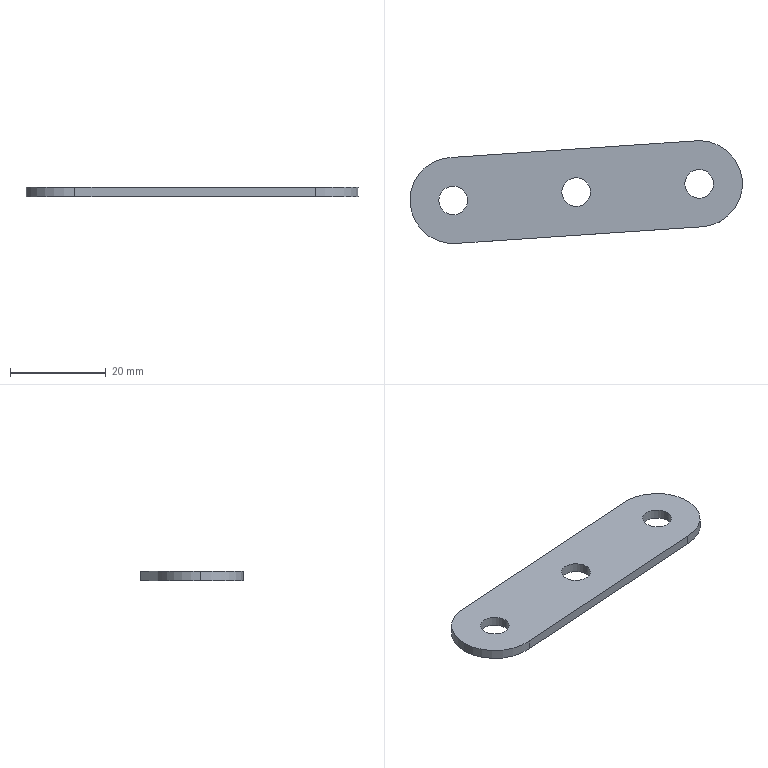Part | SolidWorks | features Extrusion 1 | 1 solid | 13 faces | box 69.294 x 21.478 x 2 mm | volume 2186 mm3 | cylinder 9 | plane 4 | commonest cylinder face diameters 6 x6 18 x3
STEP:
#1=CARTESIAN_POINT('',(-28.647,-1.739,2.));
#2=VERTEX_POINT('',#1);
#3=CARTESIAN_POINT('',(-22.647,-1.739,2.));
#4=VERTEX_POINT('',#3);
#5=CARTESIAN_POINT('',(-25.647,-1.739,2.));
#6=DIRECTION('',(0.,0.,1.));
#7=DIRECTION('',(1.,0.,0.));
#8=AXIS2_PLACEMENT_3D('',#5,#6,#7);
#9=CIRCLE('',#8,3.);
#10=EDGE_CURVE('',#2,#4,#9,.T.);
#11=ORIENTED_EDGE('',*,*,#10,.T.);
#12=CARTESIAN_POINT('',(-22.647,-1.739,0.));
#13=VERTEX_POINT('',#12);
#14=CARTESIAN_POINT('',(-22.647,-1.739,2.));
#15=DIRECTION('',(0.,0.,-1.));
#16=VECTOR('',#15,1000.);
#17=LINE('',#14,#16);
#18=EDGE_CURVE('',#4,#13,#17,.T.);
#19=ORIENTED_EDGE('',*,*,#18,.T.);
#20=CARTESIAN_POINT('',(-28.647,-1.739,0.));
#21=VERTEX_POINT('',#20);
#22=CARTESIAN_POINT('',(-25.647,-1.739,0.));
#23=DIRECTION('',(0.,0.,1.));
#24=DIRECTION('',(1.,0.,0.));
#25=AXIS2_PLACEMENT_3D('',#22,#23,#24);
#26=CIRCLE('',#25,3.);
#27=EDGE_CURVE('',#21,#13,#26,.T.);
#28=ORIENTED_EDGE('',*,*,#27,.F.);
#29=CARTESIAN_POINT('',(-28.647,-1.739,2.));
#30=DIRECTION('',(0.,0.,-1.));
#31=VECTOR('',#30,1000.);
#32=LINE('',#29,#31);
#33=EDGE_CURVE('',#2,#21,#32,.T.);
#34=ORIENTED_EDGE('',*,*,#33,.F.);
#35=EDGE_LOOP('',(#11,#19,#28,#34));
#36=FACE_OUTER_BOUND('',#35,.T.);
#37=CARTESIAN_POINT('',(-25.647,-1.739,2.));
#38=DIRECTION('',(0.,0.,-1.));
#39=DIRECTION('',(-1.,0.,0.));
#40=AXIS2_PLACEMENT_3D('',#37,#38,#39);
#41=CYLINDRICAL_SURFACE('',#40,3.);
#42=ADVANCED_FACE('',(#36),#41,.F.);
#43=CARTESIAN_POINT('',(-3.,0.,2.));
#44=VERTEX_POINT('',#43);
#45=CARTESIAN_POINT('',(3.,0.,2.));
#46=VERTEX_POINT('',#45);
#47=CARTESIAN_POINT('',(0.,0.,2.));
#48=DIRECTION('',(0.,0.,1.));
#49=DIRECTION('',(1.,0.,0.));
#50=AXIS2_PLACEMENT_3D('',#47,#48,#49);
#51=CIRCLE('',#50,3.);
#52=EDGE_CURVE('',#44,#46,#51,.T.);
#53=ORIENTED_EDGE('',*,*,#52,.T.);
#54=CARTESIAN_POINT('',(3.,0.,0.));
#55=VERTEX_POINT('',#54);
#56=CARTESIAN_POINT('',(3.,0.,2.));
#57=DIRECTION('',(0.,0.,-1.));
#58=VECTOR('',#57,1000.);
#59=LINE('',#56,#58);
#60=EDGE_CURVE('',#46,#55,#59,.T.);
#61=ORIENTED_EDGE('',*,*,#60,.T.);
#62=CARTESIAN_POINT('',(-3.,0.,0.));
#63=VERTEX_POINT('',#62);
#64=CARTESIAN_POINT('',(0.,0.,0.));
#65=DIRECTION('',(0.,0.,1.));
#66=DIRECTION('',(1.,0.,0.));
#67=AXIS2_PLACEMENT_3D('',#64,#65,#66);
#68=CIRCLE('',#67,3.);
#69=EDGE_CURVE('',#63,#55,#68,.T.);
#70=ORIENTED_EDGE('',*,*,#69,.F.);
#71=CARTESIAN_POINT('',(-3.,0.,2.));
#72=DIRECTION('',(0.,0.,-1.));
#73=VECTOR('',#72,1000.);
#74=LINE('',#71,#73);
#75=EDGE_CURVE('',#44,#63,#74,.T.);
#76=ORIENTED_EDGE('',*,*,#75,.F.);
#77=EDGE_LOOP('',(#53,#61,#70,#76));
#78=FACE_OUTER_BOUND('',#77,.T.);
#79=CARTESIAN_POINT('',(0.,0.,2.));
#80=DIRECTION('',(0.,0.,-1.));
#81=DIRECTION('',(-1.,0.,0.));
#82=AXIS2_PLACEMENT_3D('',#79,#80,#81);
#83=CYLINDRICAL_SURFACE('',#82,3.);
#84=ADVANCED_FACE('',(#78),#83,.F.);
#85=CARTESIAN_POINT('',(-54.294,-3.478,2.));
#86=VERTEX_POINT('',#85);
#87=CARTESIAN_POINT('',(-48.294,-3.478,2.));
#88=VERTEX_POINT('',#87);
#89=CARTESIAN_POINT('',(-51.294,-3.478,2.));
#90=DIRECTION('',(0.,0.,1.));
#91=DIRECTION('',(1.,0.,0.));
#92=AXIS2_PLACEMENT_3D('',#89,#90,#91);
#93=CIRCLE('',#92,3.);
#94=EDGE_CURVE('',#86,#88,#93,.T.);
#95=ORIENTED_EDGE('',*,*,#94,.T.);
#96=CARTESIAN_POINT('',(-48.294,-3.478,0.));
#97=VERTEX_POINT('',#96);
#98=CARTESIAN_POINT('',(-48.294,-3.478,2.));
#99=DIRECTION('',(0.,0.,-1.));
#100=VECTOR('',#99,1000.);
#101=LINE('',#98,#100);
#102=EDGE_CURVE('',#88,#97,#101,.T.);
#103=ORIENTED_EDGE('',*,*,#102,.T.);
#104=CARTESIAN_POINT('',(-54.294,-3.478,0.));
#105=VERTEX_POINT('',#104);
#106=CARTESIAN_POINT('',(-51.294,-3.478,0.));
#107=DIRECTION('',(0.,0.,1.));
#108=DIRECTION('',(1.,0.,0.));
#109=AXIS2_PLACEMENT_3D('',#106,#107,#108);
#110=CIRCLE('',#109,3.);
#111=EDGE_CURVE('',#105,#97,#110,.T.);
#112=ORIENTED_EDGE('',*,*,#111,.F.);
#113=CARTESIAN_POINT('',(-54.294,-3.478,2.));
#114=DIRECTION('',(0.,0.,-1.));
#115=VECTOR('',#114,1000.);
#116=LINE('',#113,#115);
#117=EDGE_CURVE('',#86,#105,#116,.T.);
#118=ORIENTED_EDGE('',*,*,#117,.F.);
#119=EDGE_LOOP('',(#95,#103,#112,#118));
#120=FACE_OUTER_BOUND('',#119,.T.);
#121=CARTESIAN_POINT('',(-51.294,-3.478,2.));
#122=DIRECTION('',(0.,0.,-1.));
#123=DIRECTION('',(-1.,0.,0.));
#124=AXIS2_PLACEMENT_3D('',#121,#122,#123);
#125=CYLINDRICAL_SURFACE('',#124,3.);
#126=ADVANCED_FACE('',(#120),#125,.F.);
#127=CARTESIAN_POINT('',(-60.294,-3.478,2.));
#128=VERTEX_POINT('',#127);
#129=CARTESIAN_POINT('',(-50.079,-12.396,2.));
#130=VERTEX_POINT('',#129);
#131=CARTESIAN_POINT('',(-51.294,-3.478,2.));
#132=DIRECTION('',(0.,0.,1.));
#133=DIRECTION('',(1.,0.,0.));
#134=AXIS2_PLACEMENT_3D('',#131,#132,#133);
#135=CIRCLE('',#134,9.);
#136=EDGE_CURVE('',#128,#130,#135,.T.);
#137=ORIENTED_EDGE('',*,*,#136,.F.);
#138=CARTESIAN_POINT('',(-60.294,-3.478,0.));
#139=VERTEX_POINT('',#138);
#140=CARTESIAN_POINT('',(-60.294,-3.478,2.));
#141=DIRECTION('',(0.,0.,-1.));
#142=VECTOR('',#141,1000.);
#143=LINE('',#140,#142);
#144=EDGE_CURVE('',#128,#139,#143,.T.);
#145=ORIENTED_EDGE('',*,*,#144,.T.);
#146=CARTESIAN_POINT('',(-50.079,-12.396,0.));
#147=VERTEX_POINT('',#146);
#148=CARTESIAN_POINT('',(-51.294,-3.478,0.));
#149=DIRECTION('',(0.,0.,1.));
#150=DIRECTION('',(1.,0.,0.));
#151=AXIS2_PLACEMENT_3D('',#148,#149,#150);
#152=CIRCLE('',#151,9.);
#153=EDGE_CURVE('',#139,#147,#152,.T.);
#154=ORIENTED_EDGE('',*,*,#153,.T.);
#155=CARTESIAN_POINT('',(-50.079,-12.396,2.));
#156=DIRECTION('',(0.,0.,-1.));
#157=VECTOR('',#156,1000.);
#158=LINE('',#155,#157);
#159=EDGE_CURVE('',#130,#147,#158,.T.);
#160=ORIENTED_EDGE('',*,*,#159,.F.);
#161=EDGE_LOOP('',(#137,#145,#154,#160));
#162=FACE_OUTER_BOUND('',#161,.T.);
#163=CARTESIAN_POINT('',(-51.294,-3.478,2.));
#164=DIRECTION('',(0.,0.,-1.));
#165=DIRECTION('',(-1.,0.,0.));
#166=AXIS2_PLACEMENT_3D('',#163,#164,#165);
#167=CYLINDRICAL_SURFACE('',#166,9.);
#168=ADVANCED_FACE('',(#162),#167,.T.);
#169=ORIENTED_EDGE('',*,*,#52,.F.);
#170=CARTESIAN_POINT('',(0.,0.,2.));
#171=DIRECTION('',(0.,0.,1.));
#172=DIRECTION('',(1.,0.,0.));
#173=AXIS2_PLACEMENT_3D('',#170,#171,#172);
#174=CIRCLE('',#173,3.);
#175=EDGE_CURVE('',#46,#44,#174,.T.);
#176=ORIENTED_EDGE('',*,*,#175,.F.);
#177=EDGE_LOOP('',(#169,#176));
#178=FACE_BOUND('',#177,.T.);
#179=CARTESIAN_POINT('',(-51.294,5.522,2.));
#180=VERTEX_POINT('',#179);
#181=CARTESIAN_POINT('',(-51.294,-3.478,2.));
#182=DIRECTION('',(0.,0.,1.));
#183=DIRECTION('',(1.,0.,0.));
#184=AXIS2_PLACEMENT_3D('',#181,#182,#183);
#185=CIRCLE('',#184,9.);
#186=EDGE_CURVE('',#180,#128,#185,.T.);
#187=ORIENTED_EDGE('',*,*,#186,.T.);
#188=ORIENTED_EDGE('',*,*,#136,.T.);
#189=CARTESIAN_POINT('',(0.,-9.,2.));
#190=VERTEX_POINT('',#189);
#191=CARTESIAN_POINT('',(-50.079,-12.396,2.));
#192=DIRECTION('',(0.9977,0.06765,0.));
#193=VECTOR('',#192,1000.);
#194=LINE('',#191,#193);
#195=EDGE_CURVE('',#130,#190,#194,.T.);
#196=ORIENTED_EDGE('',*,*,#195,.T.);
#197=CARTESIAN_POINT('',(0.,9.,2.));
#198=VERTEX_POINT('',#197);
#199=CARTESIAN_POINT('',(0.,0.,2.));
#200=DIRECTION('',(0.,0.,1.));
#201=DIRECTION('',(1.,0.,0.));
#202=AXIS2_PLACEMENT_3D('',#199,#200,#201);
#203=CIRCLE('',#202,9.);
#204=EDGE_CURVE('',#190,#198,#203,.T.);
#205=ORIENTED_EDGE('',*,*,#204,.T.);
#206=CARTESIAN_POINT('',(-51.294,5.522,2.));
#207=DIRECTION('',(-0.9977,-0.06765,0.));
#208=VECTOR('',#207,1000.);
#209=LINE('',#206,#208);
#210=EDGE_CURVE('',#198,#180,#209,.T.);
#211=ORIENTED_EDGE('',*,*,#210,.T.);
#212=EDGE_LOOP('',(#187,#188,#196,#205,#211));
#213=FACE_OUTER_BOUND('',#212,.T.);
#214=ORIENTED_EDGE('',*,*,#94,.F.);
#215=CARTESIAN_POINT('',(-51.294,-3.478,2.));
#216=DIRECTION('',(0.,0.,1.));
#217=DIRECTION('',(1.,0.,0.));
#218=AXIS2_PLACEMENT_3D('',#215,#216,#217);
#219=CIRCLE('',#218,3.);
#220=EDGE_CURVE('',#88,#86,#219,.T.);
#221=ORIENTED_EDGE('',*,*,#220,.F.);
#222=EDGE_LOOP('',(#214,#221));
#223=FACE_BOUND('',#222,.T.);
#224=ORIENTED_EDGE('',*,*,#10,.F.);
#225=CARTESIAN_POINT('',(-25.647,-1.739,2.));
#226=DIRECTION('',(0.,0.,1.));
#227=DIRECTION('',(1.,0.,0.));
#228=AXIS2_PLACEMENT_3D('',#225,#226,#227);
#229=CIRCLE('',#228,3.);
#230=EDGE_CURVE('',#4,#2,#229,.T.);
#231=ORIENTED_EDGE('',*,*,#230,.F.);
#232=EDGE_LOOP('',(#224,#231));
#233=FACE_BOUND('',#232,.T.);
#234=CARTESIAN_POINT('',(-51.294,-3.478,2.));
#235=DIRECTION('',(0.,0.,1.));
#236=DIRECTION('',(1.,0.,0.));
#237=AXIS2_PLACEMENT_3D('',#234,#235,#236);
#238=PLANE('',#237);
#239=ADVANCED_FACE('',(#178,#213,#223,#233),#238,.T.);
#240=CARTESIAN_POINT('',(-51.294,5.522,0.));
#241=VERTEX_POINT('',#240);
#242=CARTESIAN_POINT('',(-51.294,-3.478,0.));
#243=DIRECTION('',(0.,0.,1.));
#244=DIRECTION('',(1.,0.,0.));
#245=AXIS2_PLACEMENT_3D('',#242,#243,#244);
#246=CIRCLE('',#245,9.);
#247=EDGE_CURVE('',#241,#139,#246,.T.);
#248=ORIENTED_EDGE('',*,*,#247,.F.);
#249=CARTESIAN_POINT('',(0.,9.,0.));
#250=VERTEX_POINT('',#249);
#251=CARTESIAN_POINT('',(-51.294,5.522,0.));
#252=DIRECTION('',(-0.9977,-0.06765,0.));
#253=VECTOR('',#252,1000.);
#254=LINE('',#251,#253);
#255=EDGE_CURVE('',#250,#241,#254,.T.);
#256=ORIENTED_EDGE('',*,*,#255,.F.);
#257=CARTESIAN_POINT('',(0.,-9.,0.));
#258=VERTEX_POINT('',#257);
#259=CARTESIAN_POINT('',(0.,0.,0.));
#260=DIRECTION('',(0.,0.,1.));
#261=DIRECTION('',(1.,0.,0.));
#262=AXIS2_PLACEMENT_3D('',#259,#260,#261);
#263=CIRCLE('',#262,9.);
#264=EDGE_CURVE('',#258,#250,#263,.T.);
#265=ORIENTED_EDGE('',*,*,#264,.F.);
#266=CARTESIAN_POINT('',(-50.079,-12.396,0.));
#267=DIRECTION('',(0.9977,0.06765,0.));
#268=VECTOR('',#267,1000.);
#269=LINE('',#266,#268);
#270=EDGE_CURVE('',#147,#258,#269,.T.);
#271=ORIENTED_EDGE('',*,*,#270,.F.);
#272=ORIENTED_EDGE('',*,*,#153,.F.);
#273=EDGE_LOOP('',(#248,#256,#265,#271,#272));
#274=FACE_OUTER_BOUND('',#273,.T.);
#275=ORIENTED_EDGE('',*,*,#111,.T.);
#276=CARTESIAN_POINT('',(-51.294,-3.478,0.));
#277=DIRECTION('',(0.,0.,1.));
#278=DIRECTION('',(1.,0.,0.));
#279=AXIS2_PLACEMENT_3D('',#276,#277,#278);
#280=CIRCLE('',#279,3.);
#281=EDGE_CURVE('',#97,#105,#280,.T.);
#282=ORIENTED_EDGE('',*,*,#281,.T.);
#283=EDGE_LOOP('',(#275,#282));
#284=FACE_BOUND('',#283,.T.);
#285=ORIENTED_EDGE('',*,*,#69,.T.);
#286=CARTESIAN_POINT('',(0.,0.,0.));
#287=DIRECTION('',(0.,0.,1.));
#288=DIRECTION('',(1.,0.,0.));
#289=AXIS2_PLACEMENT_3D('',#286,#287,#288);
#290=CIRCLE('',#289,3.);
#291=EDGE_CURVE('',#55,#63,#290,.T.);
#292=ORIENTED_EDGE('',*,*,#291,.T.);
#293=EDGE_LOOP('',(#285,#292));
#294=FACE_BOUND('',#293,.T.);
#295=ORIENTED_EDGE('',*,*,#27,.T.);
#296=CARTESIAN_POINT('',(-25.647,-1.739,0.));
#297=DIRECTION('',(0.,0.,1.));
#298=DIRECTION('',(1.,0.,0.));
#299=AXIS2_PLACEMENT_3D('',#296,#297,#298);
#300=CIRCLE('',#299,3.);
#301=EDGE_CURVE('',#13,#21,#300,.T.);
#302=ORIENTED_EDGE('',*,*,#301,.T.);
#303=EDGE_LOOP('',(#295,#302));
#304=FACE_BOUND('',#303,.T.);
#305=CARTESIAN_POINT('',(-51.294,-3.478,0.));
#306=DIRECTION('',(0.,0.,1.));
#307=DIRECTION('',(1.,0.,0.));
#308=AXIS2_PLACEMENT_3D('',#305,#306,#307);
#309=PLANE('',#308);
#310=ADVANCED_FACE('',(#274,#284,#294,#304),#309,.F.);
#311=ORIENTED_EDGE('',*,*,#144,.F.);
#312=ORIENTED_EDGE('',*,*,#186,.F.);
#313=CARTESIAN_POINT('',(-51.294,5.522,2.));
#314=DIRECTION('',(0.,0.,-1.));
#315=VECTOR('',#314,1000.);
#316=LINE('',#313,#315);
#317=EDGE_CURVE('',#180,#241,#316,.T.);
#318=ORIENTED_EDGE('',*,*,#317,.T.);
#319=ORIENTED_EDGE('',*,*,#247,.T.);
#320=EDGE_LOOP('',(#311,#312,#318,#319));
#321=FACE_OUTER_BOUND('',#320,.T.);
#322=CARTESIAN_POINT('',(-51.294,-3.478,2.));
#323=DIRECTION('',(0.,0.,-1.));
#324=DIRECTION('',(-1.,0.,0.));
#325=AXIS2_PLACEMENT_3D('',#322,#323,#324);
#326=CYLINDRICAL_SURFACE('',#325,9.);
#327=ADVANCED_FACE('',(#321),#326,.T.);
#328=ORIENTED_EDGE('',*,*,#270,.T.);
#329=CARTESIAN_POINT('',(0.,-9.,2.));
#330=DIRECTION('',(0.,0.,-1.));
#331=VECTOR('',#330,1000.);
#332=LINE('',#329,#331);
#333=EDGE_CURVE('',#190,#258,#332,.T.);
#334=ORIENTED_EDGE('',*,*,#333,.F.);
#335=ORIENTED_EDGE('',*,*,#195,.F.);
#336=ORIENTED_EDGE('',*,*,#159,.T.);
#337=EDGE_LOOP('',(#328,#334,#335,#336));
#338=FACE_OUTER_BOUND('',#337,.T.);
#339=CARTESIAN_POINT('',(-50.079,-12.396,2.));
#340=DIRECTION('',(-0.06765,0.9977,0.));
#341=DIRECTION('',(-0.9977,-0.06765,0.));
#342=AXIS2_PLACEMENT_3D('',#339,#340,#341);
#343=PLANE('',#342);
#344=ADVANCED_FACE('',(#338),#343,.F.);
#345=ORIENTED_EDGE('',*,*,#264,.T.);
#346=CARTESIAN_POINT('',(0.,9.,2.));
#347=DIRECTION('',(0.,0.,-1.));
#348=VECTOR('',#347,1000.);
#349=LINE('',#346,#348);
#350=EDGE_CURVE('',#198,#250,#349,.T.);
#351=ORIENTED_EDGE('',*,*,#350,.F.);
#352=ORIENTED_EDGE('',*,*,#204,.F.);
#353=ORIENTED_EDGE('',*,*,#333,.T.);
#354=EDGE_LOOP('',(#345,#351,#352,#353));
#355=FACE_OUTER_BOUND('',#354,.T.);
#356=CARTESIAN_POINT('',(0.,0.,2.));
#357=DIRECTION('',(0.,0.,-1.));
#358=DIRECTION('',(-1.,0.,0.));
#359=AXIS2_PLACEMENT_3D('',#356,#357,#358);
#360=CYLINDRICAL_SURFACE('',#359,9.);
#361=ADVANCED_FACE('',(#355),#360,.T.);
#362=ORIENTED_EDGE('',*,*,#255,.T.);
#363=ORIENTED_EDGE('',*,*,#317,.F.);
#364=ORIENTED_EDGE('',*,*,#210,.F.);
#365=ORIENTED_EDGE('',*,*,#350,.T.);
#366=EDGE_LOOP('',(#362,#363,#364,#365));
#367=FACE_OUTER_BOUND('',#366,.T.);
#368=CARTESIAN_POINT('',(-51.294,5.522,2.));
#369=DIRECTION('',(0.06765,-0.9977,0.));
#370=DIRECTION('',(0.9977,0.06765,0.));
#371=AXIS2_PLACEMENT_3D('',#368,#369,#370);
#372=PLANE('',#371);
#373=ADVANCED_FACE('',(#367),#372,.F.);
#374=ORIENTED_EDGE('',*,*,#102,.F.);
#375=ORIENTED_EDGE('',*,*,#220,.T.);
#376=ORIENTED_EDGE('',*,*,#117,.T.);
#377=ORIENTED_EDGE('',*,*,#281,.F.);
#378=EDGE_LOOP('',(#374,#375,#376,#377));
#379=FACE_OUTER_BOUND('',#378,.T.);
#380=CARTESIAN_POINT('',(-51.294,-3.478,2.));
#381=DIRECTION('',(0.,0.,-1.));
#382=DIRECTION('',(-1.,0.,0.));
#383=AXIS2_PLACEMENT_3D('',#380,#381,#382);
#384=CYLINDRICAL_SURFACE('',#383,3.);
#385=ADVANCED_FACE('',(#379),#384,.F.);
#386=ORIENTED_EDGE('',*,*,#60,.F.);
#387=ORIENTED_EDGE('',*,*,#175,.T.);
#388=ORIENTED_EDGE('',*,*,#75,.T.);
#389=ORIENTED_EDGE('',*,*,#291,.F.);
#390=EDGE_LOOP('',(#386,#387,#388,#389));
#391=FACE_OUTER_BOUND('',#390,.T.);
#392=CARTESIAN_POINT('',(0.,0.,2.));
#393=DIRECTION('',(0.,0.,-1.));
#394=DIRECTION('',(-1.,0.,0.));
#395=AXIS2_PLACEMENT_3D('',#392,#393,#394);
#396=CYLINDRICAL_SURFACE('',#395,3.);
#397=ADVANCED_FACE('',(#391),#396,.F.);
#398=ORIENTED_EDGE('',*,*,#18,.F.);
#399=ORIENTED_EDGE('',*,*,#230,.T.);
#400=ORIENTED_EDGE('',*,*,#33,.T.);
#401=ORIENTED_EDGE('',*,*,#301,.F.);
#402=EDGE_LOOP('',(#398,#399,#400,#401));
#403=FACE_OUTER_BOUND('',#402,.T.);
#404=CARTESIAN_POINT('',(-25.647,-1.739,2.));
#405=DIRECTION('',(0.,0.,-1.));
#406=DIRECTION('',(-1.,0.,0.));
#407=AXIS2_PLACEMENT_3D('',#404,#405,#406);
#408=CYLINDRICAL_SURFACE('',#407,3.);
#409=ADVANCED_FACE('',(#403),#408,.F.);
#410=CLOSED_SHELL('',(#42,#84,#126,#168,#239,#310,#327,#344,#361,#373,#385,#397,#409));
#411=MANIFOLD_SOLID_BREP('',#410);
#412=CARTESIAN_POINT('',(0.,0.,0.));
#413=DIRECTION('',(0.,0.,1.));
#414=DIRECTION('',(1.,0.,0.));
#415=AXIS2_PLACEMENT_3D('',#412,#413,#414);
#416=(LENGTH_UNIT()NAMED_UNIT(*)SI_UNIT(.MILLI.,.METRE.));
#417=UNCERTAINTY_MEASURE_WITH_UNIT(LENGTH_MEASURE(0.00001),#416,'','');
#418=(NAMED_UNIT(*)PLANE_ANGLE_UNIT()SI_UNIT($,.RADIAN.));
#419=(NAMED_UNIT(*)SI_UNIT($,.STERADIAN.)SOLID_ANGLE_UNIT());
#420=(GEOMETRIC_REPRESENTATION_CONTEXT(3)GLOBAL_UNCERTAINTY_ASSIGNED_CONTEXT((#417))GLOBAL_UNIT_ASSIGNED_CONTEXT((#416,#418,#419))REPRESENTATION_CONTEXT('',''));
#421=ADVANCED_BREP_SHAPE_REPRESENTATION('',(#411,#415),#420);